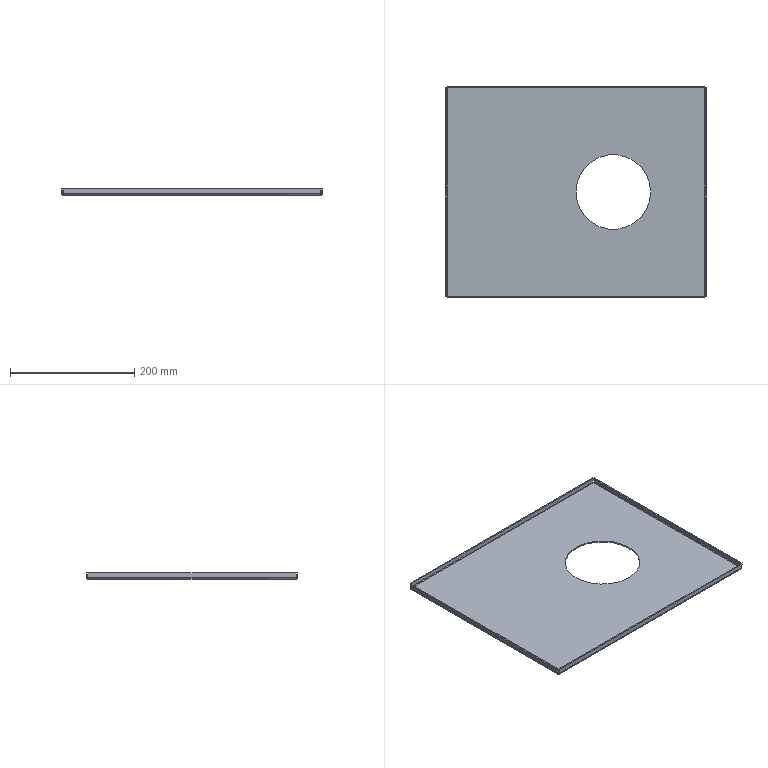Part | SolidWorks | features BaseBody 1 | 1 solid | 40 faces | box 420 x 340 x 10 mm | volume 284661 mm3 | plane 22 | cylinder 10 | spline 8 | commonest cylinder face diameters 1.473 x4 5.473 x4 120 x2